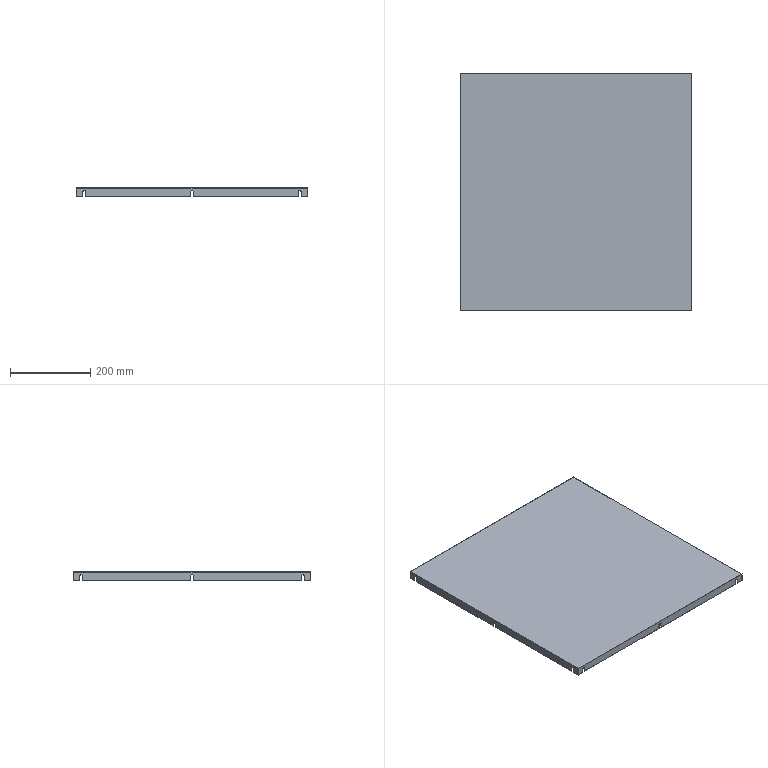Part | STEP file | 1 solid | 64 faces | box 578 x 593 x 20 mm | volume 386105 mm3 | plane 46 | cylinder 18 | commonest cylinder face diameters 7 x18